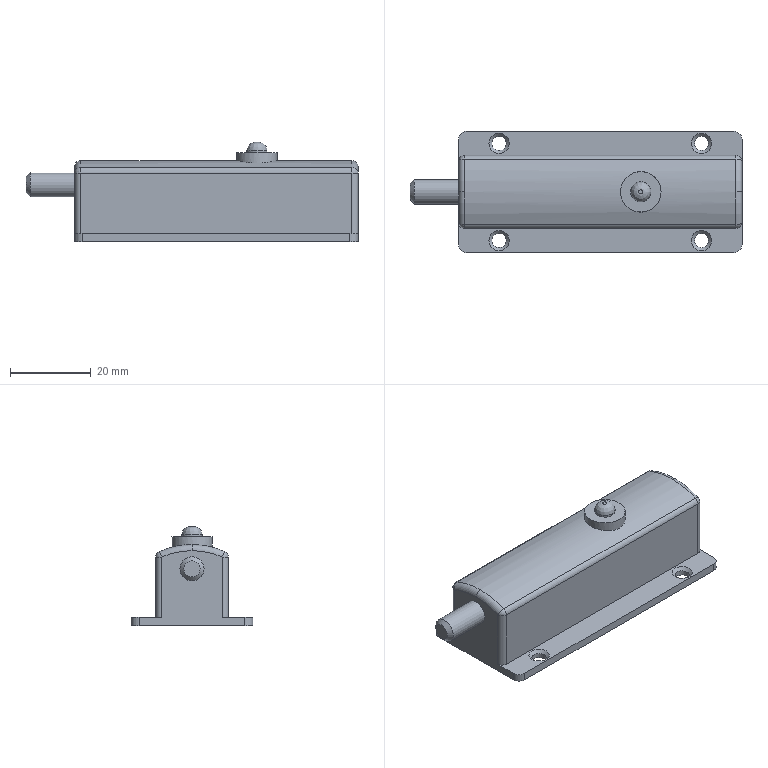Part | STEP file | Frame_top | 1 solid | 44 faces | box 82 x 30 x 24.5 mm | volume 26373 mm3 | cylinder 18 | plane 12 | cone 5 | torus 4 | sphere 4 | other 1 | commonest cylinder face diameters 3 x6 3.5 x4 4 x4 5 x1 6 x1 10 x1